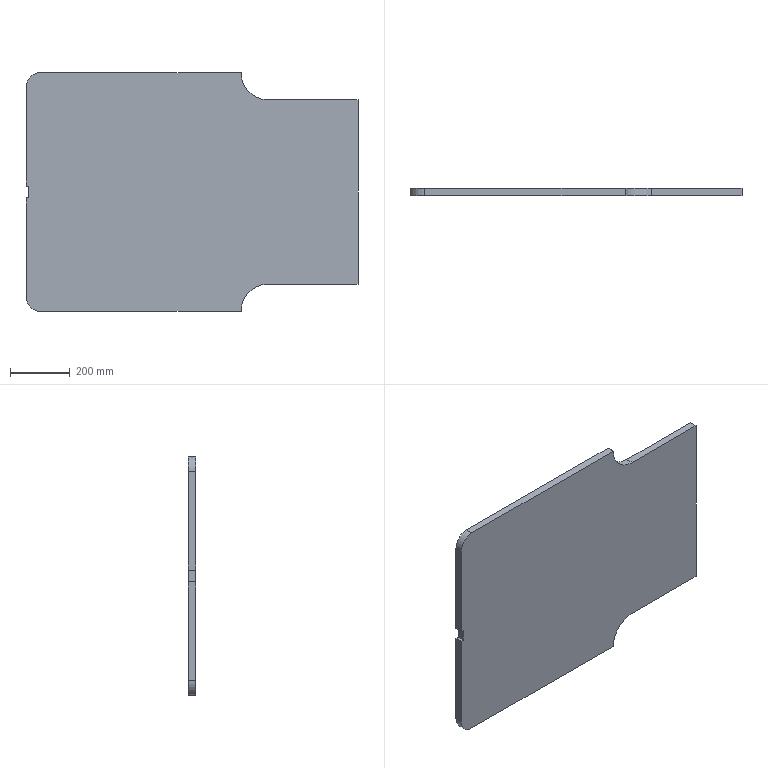Part | SolidWorks | features BaseBody 1 | 1 solid | 54 faces | box 1112 x 25 x 800 mm | volume 20489758 mm3 | cylinder 28 | plane 26 | commonest cylinder face diameters 10 x24 100 x2 178 x2
STEP:
#1=CARTESIAN_POINT('',(-375.282,-2.862,-275.));
#2=VERTEX_POINT('',#1);
#3=CARTESIAN_POINT('',(-375.282,-2.862,-265.));
#4=VERTEX_POINT('',#3);
#5=CARTESIAN_POINT('',(-375.282,-2.862,-270.));
#6=DIRECTION('',(0.,1.,0.));
#7=DIRECTION('',(0.,0.,1.));
#8=AXIS2_PLACEMENT_3D('',#5,#6,#7);
#9=CIRCLE('',#8,5.);
#10=EDGE_CURVE('',#2,#4,#9,.T.);
#11=ORIENTED_EDGE('',*,*,#10,.F.);
#12=CARTESIAN_POINT('',(-375.282,7.138,-275.));
#13=VERTEX_POINT('',#12);
#14=CARTESIAN_POINT('',(-375.282,-2.862,-275.));
#15=DIRECTION('',(0.,1.,0.));
#16=VECTOR('',#15,1000.);
#17=LINE('',#14,#16);
#18=EDGE_CURVE('',#2,#13,#17,.T.);
#19=ORIENTED_EDGE('',*,*,#18,.T.);
#20=CARTESIAN_POINT('',(-375.282,7.138,-265.));
#21=VERTEX_POINT('',#20);
#22=CARTESIAN_POINT('',(-375.282,7.138,-270.));
#23=DIRECTION('',(0.,-1.,0.));
#24=DIRECTION('',(0.,0.,1.));
#25=AXIS2_PLACEMENT_3D('',#22,#23,#24);
#26=CIRCLE('',#25,5.);
#27=EDGE_CURVE('',#21,#13,#26,.T.);
#28=ORIENTED_EDGE('',*,*,#27,.F.);
#29=CARTESIAN_POINT('',(-375.282,-2.862,-265.));
#30=DIRECTION('',(0.,1.,0.));
#31=VECTOR('',#30,1000.);
#32=LINE('',#29,#31);
#33=EDGE_CURVE('',#4,#21,#32,.T.);
#34=ORIENTED_EDGE('',*,*,#33,.F.);
#35=EDGE_LOOP('',(#11,#19,#28,#34));
#36=FACE_OUTER_BOUND('',#35,.T.);
#37=CARTESIAN_POINT('',(-375.282,-2.862,-270.));
#38=DIRECTION('',(0.,1.,0.));
#39=DIRECTION('',(0.,0.,1.));
#40=AXIS2_PLACEMENT_3D('',#37,#38,#39);
#41=CYLINDRICAL_SURFACE('',#40,5.);
#42=ADVANCED_FACE('',(#36),#41,.F.);
#43=CARTESIAN_POINT('',(-510.782,-2.862,-275.));
#44=VERTEX_POINT('',#43);
#45=CARTESIAN_POINT('',(-510.782,-2.862,-265.));
#46=VERTEX_POINT('',#45);
#47=CARTESIAN_POINT('',(-510.782,-2.862,-270.));
#48=DIRECTION('',(0.,1.,0.));
#49=DIRECTION('',(0.,0.,1.));
#50=AXIS2_PLACEMENT_3D('',#47,#48,#49);
#51=CIRCLE('',#50,5.);
#52=EDGE_CURVE('',#44,#46,#51,.T.);
#53=ORIENTED_EDGE('',*,*,#52,.F.);
#54=CARTESIAN_POINT('',(-510.782,7.138,-275.));
#55=VERTEX_POINT('',#54);
#56=CARTESIAN_POINT('',(-510.782,-2.862,-275.));
#57=DIRECTION('',(0.,1.,0.));
#58=VECTOR('',#57,1000.);
#59=LINE('',#56,#58);
#60=EDGE_CURVE('',#44,#55,#59,.T.);
#61=ORIENTED_EDGE('',*,*,#60,.T.);
#62=CARTESIAN_POINT('',(-510.782,7.138,-265.));
#63=VERTEX_POINT('',#62);
#64=CARTESIAN_POINT('',(-510.782,7.138,-270.));
#65=DIRECTION('',(0.,-1.,0.));
#66=DIRECTION('',(0.,0.,1.));
#67=AXIS2_PLACEMENT_3D('',#64,#65,#66);
#68=CIRCLE('',#67,5.);
#69=EDGE_CURVE('',#63,#55,#68,.T.);
#70=ORIENTED_EDGE('',*,*,#69,.F.);
#71=CARTESIAN_POINT('',(-510.782,-2.862,-265.));
#72=DIRECTION('',(0.,1.,0.));
#73=VECTOR('',#72,1000.);
#74=LINE('',#71,#73);
#75=EDGE_CURVE('',#46,#63,#74,.T.);
#76=ORIENTED_EDGE('',*,*,#75,.F.);
#77=EDGE_LOOP('',(#53,#61,#70,#76));
#78=FACE_OUTER_BOUND('',#77,.T.);
#79=CARTESIAN_POINT('',(-510.782,-2.862,-270.));
#80=DIRECTION('',(0.,1.,0.));
#81=DIRECTION('',(0.,0.,1.));
#82=AXIS2_PLACEMENT_3D('',#79,#80,#81);
#83=CYLINDRICAL_SURFACE('',#82,5.);
#84=ADVANCED_FACE('',(#78),#83,.F.);
#85=CARTESIAN_POINT('',(418.218,-2.862,-285.));
#86=VERTEX_POINT('',#85);
#87=CARTESIAN_POINT('',(418.218,-2.862,-275.));
#88=VERTEX_POINT('',#87);
#89=CARTESIAN_POINT('',(418.218,-2.862,-280.));
#90=DIRECTION('',(0.,1.,0.));
#91=DIRECTION('',(0.,0.,1.));
#92=AXIS2_PLACEMENT_3D('',#89,#90,#91);
#93=CIRCLE('',#92,5.);
#94=EDGE_CURVE('',#86,#88,#93,.T.);
#95=ORIENTED_EDGE('',*,*,#94,.F.);
#96=CARTESIAN_POINT('',(418.218,7.138,-285.));
#97=VERTEX_POINT('',#96);
#98=CARTESIAN_POINT('',(418.218,-2.862,-285.));
#99=DIRECTION('',(0.,1.,0.));
#100=VECTOR('',#99,1000.);
#101=LINE('',#98,#100);
#102=EDGE_CURVE('',#86,#97,#101,.T.);
#103=ORIENTED_EDGE('',*,*,#102,.T.);
#104=CARTESIAN_POINT('',(418.218,7.138,-275.));
#105=VERTEX_POINT('',#104);
#106=CARTESIAN_POINT('',(418.218,7.138,-280.));
#107=DIRECTION('',(0.,-1.,0.));
#108=DIRECTION('',(0.,0.,1.));
#109=AXIS2_PLACEMENT_3D('',#106,#107,#108);
#110=CIRCLE('',#109,5.);
#111=EDGE_CURVE('',#105,#97,#110,.T.);
#112=ORIENTED_EDGE('',*,*,#111,.F.);
#113=CARTESIAN_POINT('',(418.218,-2.862,-275.));
#114=DIRECTION('',(0.,1.,0.));
#115=VECTOR('',#114,1000.);
#116=LINE('',#113,#115);
#117=EDGE_CURVE('',#88,#105,#116,.T.);
#118=ORIENTED_EDGE('',*,*,#117,.F.);
#119=EDGE_LOOP('',(#95,#103,#112,#118));
#120=FACE_OUTER_BOUND('',#119,.T.);
#121=CARTESIAN_POINT('',(418.218,-2.862,-280.));
#122=DIRECTION('',(0.,1.,0.));
#123=DIRECTION('',(0.,0.,1.));
#124=AXIS2_PLACEMENT_3D('',#121,#122,#123);
#125=CYLINDRICAL_SURFACE('',#124,5.);
#126=ADVANCED_FACE('',(#120),#125,.F.);
#127=CARTESIAN_POINT('',(299.701,-2.862,-285.));
#128=VERTEX_POINT('',#127);
#129=CARTESIAN_POINT('',(299.701,-2.862,-275.));
#130=VERTEX_POINT('',#129);
#131=CARTESIAN_POINT('',(299.701,-2.862,-280.));
#132=DIRECTION('',(0.,1.,0.));
#133=DIRECTION('',(0.,0.,1.));
#134=AXIS2_PLACEMENT_3D('',#131,#132,#133);
#135=CIRCLE('',#134,5.);
#136=EDGE_CURVE('',#128,#130,#135,.T.);
#137=ORIENTED_EDGE('',*,*,#136,.F.);
#138=CARTESIAN_POINT('',(299.701,7.138,-285.));
#139=VERTEX_POINT('',#138);
#140=CARTESIAN_POINT('',(299.701,-2.862,-285.));
#141=DIRECTION('',(0.,1.,0.));
#142=VECTOR('',#141,1000.);
#143=LINE('',#140,#142);
#144=EDGE_CURVE('',#128,#139,#143,.T.);
#145=ORIENTED_EDGE('',*,*,#144,.T.);
#146=CARTESIAN_POINT('',(299.701,7.138,-275.));
#147=VERTEX_POINT('',#146);
#148=CARTESIAN_POINT('',(299.701,7.138,-280.));
#149=DIRECTION('',(0.,-1.,0.));
#150=DIRECTION('',(0.,0.,1.));
#151=AXIS2_PLACEMENT_3D('',#148,#149,#150);
#152=CIRCLE('',#151,5.);
#153=EDGE_CURVE('',#147,#139,#152,.T.);
#154=ORIENTED_EDGE('',*,*,#153,.F.);
#155=CARTESIAN_POINT('',(299.701,-2.862,-275.));
#156=DIRECTION('',(0.,1.,0.));
#157=VECTOR('',#156,1000.);
#158=LINE('',#155,#157);
#159=EDGE_CURVE('',#130,#147,#158,.T.);
#160=ORIENTED_EDGE('',*,*,#159,.F.);
#161=EDGE_LOOP('',(#137,#145,#154,#160));
#162=FACE_OUTER_BOUND('',#161,.T.);
#163=CARTESIAN_POINT('',(299.701,-2.862,-280.));
#164=DIRECTION('',(0.,1.,0.));
#165=DIRECTION('',(0.,0.,1.));
#166=AXIS2_PLACEMENT_3D('',#163,#164,#165);
#167=CYLINDRICAL_SURFACE('',#166,5.);
#168=ADVANCED_FACE('',(#162),#167,.F.);
#169=CARTESIAN_POINT('',(418.218,-2.862,275.));
#170=VERTEX_POINT('',#169);
#171=CARTESIAN_POINT('',(418.218,-2.862,285.));
#172=VERTEX_POINT('',#171);
#173=CARTESIAN_POINT('',(418.218,-2.862,280.));
#174=DIRECTION('',(0.,1.,0.));
#175=DIRECTION('',(0.,0.,-1.));
#176=AXIS2_PLACEMENT_3D('',#173,#174,#175);
#177=CIRCLE('',#176,5.);
#178=EDGE_CURVE('',#170,#172,#177,.T.);
#179=ORIENTED_EDGE('',*,*,#178,.F.);
#180=CARTESIAN_POINT('',(418.218,7.138,275.));
#181=VERTEX_POINT('',#180);
#182=CARTESIAN_POINT('',(418.218,-2.862,275.));
#183=DIRECTION('',(0.,1.,0.));
#184=VECTOR('',#183,1000.);
#185=LINE('',#182,#184);
#186=EDGE_CURVE('',#170,#181,#185,.T.);
#187=ORIENTED_EDGE('',*,*,#186,.T.);
#188=CARTESIAN_POINT('',(418.218,7.138,285.));
#189=VERTEX_POINT('',#188);
#190=CARTESIAN_POINT('',(418.218,7.138,280.));
#191=DIRECTION('',(0.,-1.,0.));
#192=DIRECTION('',(0.,0.,1.));
#193=AXIS2_PLACEMENT_3D('',#190,#191,#192);
#194=CIRCLE('',#193,5.);
#195=EDGE_CURVE('',#189,#181,#194,.T.);
#196=ORIENTED_EDGE('',*,*,#195,.F.);
#197=CARTESIAN_POINT('',(418.218,-2.862,285.));
#198=DIRECTION('',(0.,1.,0.));
#199=VECTOR('',#198,1000.);
#200=LINE('',#197,#199);
#201=EDGE_CURVE('',#172,#189,#200,.T.);
#202=ORIENTED_EDGE('',*,*,#201,.F.);
#203=EDGE_LOOP('',(#179,#187,#196,#202));
#204=FACE_OUTER_BOUND('',#203,.T.);
#205=CARTESIAN_POINT('',(418.218,-2.862,280.));
#206=DIRECTION('',(0.,1.,0.));
#207=DIRECTION('',(0.,0.,1.));
#208=AXIS2_PLACEMENT_3D('',#205,#206,#207);
#209=CYLINDRICAL_SURFACE('',#208,5.);
#210=ADVANCED_FACE('',(#204),#209,.F.);
#211=CARTESIAN_POINT('',(299.701,-2.862,275.));
#212=VERTEX_POINT('',#211);
#213=CARTESIAN_POINT('',(299.701,-2.862,285.));
#214=VERTEX_POINT('',#213);
#215=CARTESIAN_POINT('',(299.701,-2.862,280.));
#216=DIRECTION('',(0.,1.,0.));
#217=DIRECTION('',(0.,0.,-1.));
#218=AXIS2_PLACEMENT_3D('',#215,#216,#217);
#219=CIRCLE('',#218,5.);
#220=EDGE_CURVE('',#212,#214,#219,.T.);
#221=ORIENTED_EDGE('',*,*,#220,.F.);
#222=CARTESIAN_POINT('',(299.701,7.138,275.));
#223=VERTEX_POINT('',#222);
#224=CARTESIAN_POINT('',(299.701,-2.862,275.));
#225=DIRECTION('',(0.,1.,0.));
#226=VECTOR('',#225,1000.);
#227=LINE('',#224,#226);
#228=EDGE_CURVE('',#212,#223,#227,.T.);
#229=ORIENTED_EDGE('',*,*,#228,.T.);
#230=CARTESIAN_POINT('',(299.701,7.138,285.));
#231=VERTEX_POINT('',#230);
#232=CARTESIAN_POINT('',(299.701,7.138,280.));
#233=DIRECTION('',(0.,-1.,0.));
#234=DIRECTION('',(0.,0.,1.));
#235=AXIS2_PLACEMENT_3D('',#232,#233,#234);
#236=CIRCLE('',#235,5.);
#237=EDGE_CURVE('',#231,#223,#236,.T.);
#238=ORIENTED_EDGE('',*,*,#237,.F.);
#239=CARTESIAN_POINT('',(299.701,-2.862,285.));
#240=DIRECTION('',(0.,1.,0.));
#241=VECTOR('',#240,1000.);
#242=LINE('',#239,#241);
#243=EDGE_CURVE('',#214,#231,#242,.T.);
#244=ORIENTED_EDGE('',*,*,#243,.F.);
#245=EDGE_LOOP('',(#221,#229,#238,#244));
#246=FACE_OUTER_BOUND('',#245,.T.);
#247=CARTESIAN_POINT('',(299.701,-2.862,280.));
#248=DIRECTION('',(0.,1.,0.));
#249=DIRECTION('',(0.,0.,1.));
#250=AXIS2_PLACEMENT_3D('',#247,#248,#249);
#251=CYLINDRICAL_SURFACE('',#250,5.);
#252=ADVANCED_FACE('',(#246),#251,.F.);
#253=CARTESIAN_POINT('',(-375.282,-2.862,265.));
#254=VERTEX_POINT('',#253);
#255=CARTESIAN_POINT('',(-375.282,-2.862,275.));
#256=VERTEX_POINT('',#255);
#257=CARTESIAN_POINT('',(-375.282,-2.862,270.));
#258=DIRECTION('',(0.,1.,0.));
#259=DIRECTION('',(0.,0.,-1.));
#260=AXIS2_PLACEMENT_3D('',#257,#258,#259);
#261=CIRCLE('',#260,5.);
#262=EDGE_CURVE('',#254,#256,#261,.T.);
#263=ORIENTED_EDGE('',*,*,#262,.F.);
#264=CARTESIAN_POINT('',(-375.282,7.138,265.));
#265=VERTEX_POINT('',#264);
#266=CARTESIAN_POINT('',(-375.282,-2.862,265.));
#267=DIRECTION('',(0.,1.,0.));
#268=VECTOR('',#267,1000.);
#269=LINE('',#266,#268);
#270=EDGE_CURVE('',#254,#265,#269,.T.);
#271=ORIENTED_EDGE('',*,*,#270,.T.);
#272=CARTESIAN_POINT('',(-375.282,7.138,275.));
#273=VERTEX_POINT('',#272);
#274=CARTESIAN_POINT('',(-375.282,7.138,270.));
#275=DIRECTION('',(0.,-1.,0.));
#276=DIRECTION('',(0.,0.,1.));
#277=AXIS2_PLACEMENT_3D('',#274,#275,#276);
#278=CIRCLE('',#277,5.);
#279=EDGE_CURVE('',#273,#265,#278,.T.);
#280=ORIENTED_EDGE('',*,*,#279,.F.);
#281=CARTESIAN_POINT('',(-375.282,-2.862,275.));
#282=DIRECTION('',(0.,1.,0.));
#283=VECTOR('',#282,1000.);
#284=LINE('',#281,#283);
#285=EDGE_CURVE('',#256,#273,#284,.T.);
#286=ORIENTED_EDGE('',*,*,#285,.F.);
#287=EDGE_LOOP('',(#263,#271,#280,#286));
#288=FACE_OUTER_BOUND('',#287,.T.);
#289=CARTESIAN_POINT('',(-375.282,-2.862,270.));
#290=DIRECTION('',(0.,1.,0.));
#291=DIRECTION('',(0.,0.,1.));
#292=AXIS2_PLACEMENT_3D('',#289,#290,#291);
#293=CYLINDRICAL_SURFACE('',#292,5.);
#294=ADVANCED_FACE('',(#288),#293,.F.);
#295=CARTESIAN_POINT('',(-510.782,-2.862,265.));
#296=VERTEX_POINT('',#295);
#297=CARTESIAN_POINT('',(-510.782,-2.862,275.));
#298=VERTEX_POINT('',#297);
#299=CARTESIAN_POINT('',(-510.782,-2.862,270.));
#300=DIRECTION('',(0.,1.,0.));
#301=DIRECTION('',(0.,0.,-1.));
#302=AXIS2_PLACEMENT_3D('',#299,#300,#301);
#303=CIRCLE('',#302,5.);
#304=EDGE_CURVE('',#296,#298,#303,.T.);
#305=ORIENTED_EDGE('',*,*,#304,.F.);
#306=CARTESIAN_POINT('',(-510.782,7.138,265.));
#307=VERTEX_POINT('',#306);
#308=CARTESIAN_POINT('',(-510.782,-2.862,265.));
#309=DIRECTION('',(0.,1.,0.));
#310=VECTOR('',#309,1000.);
#311=LINE('',#308,#310);
#312=EDGE_CURVE('',#296,#307,#311,.T.);
#313=ORIENTED_EDGE('',*,*,#312,.T.);
#314=CARTESIAN_POINT('',(-510.782,7.138,275.));
#315=VERTEX_POINT('',#314);
#316=CARTESIAN_POINT('',(-510.782,7.138,270.));
#317=DIRECTION('',(0.,-1.,0.));
#318=DIRECTION('',(0.,0.,1.));
#319=AXIS2_PLACEMENT_3D('',#316,#317,#318);
#320=CIRCLE('',#319,5.);
#321=EDGE_CURVE('',#315,#307,#320,.T.);
#322=ORIENTED_EDGE('',*,*,#321,.F.);
#323=CARTESIAN_POINT('',(-510.782,-2.862,275.));
#324=DIRECTION('',(0.,1.,0.));
#325=VECTOR('',#324,1000.);
#326=LINE('',#323,#325);
#327=EDGE_CURVE('',#298,#315,#326,.T.);
#328=ORIENTED_EDGE('',*,*,#327,.F.);
#329=EDGE_LOOP('',(#305,#313,#322,#328));
#330=FACE_OUTER_BOUND('',#329,.T.);
#331=CARTESIAN_POINT('',(-510.782,-2.862,270.));
#332=DIRECTION('',(0.,1.,0.));
#333=DIRECTION('',(0.,0.,1.));
#334=AXIS2_PLACEMENT_3D('',#331,#332,#333);
#335=CYLINDRICAL_SURFACE('',#334,5.);
#336=ADVANCED_FACE('',(#330),#335,.F.);
#337=CARTESIAN_POINT('',(-246.782,-2.862,105.));
#338=VERTEX_POINT('',#337);
#339=CARTESIAN_POINT('',(-246.782,-2.862,115.));
#340=VERTEX_POINT('',#339);
#341=CARTESIAN_POINT('',(-246.782,-2.862,110.));
#342=DIRECTION('',(0.,1.,0.));
#343=DIRECTION('',(0.,0.,1.));
#344=AXIS2_PLACEMENT_3D('',#341,#342,#343);
#345=CIRCLE('',#344,5.);
#346=EDGE_CURVE('',#338,#340,#345,.T.);
#347=ORIENTED_EDGE('',*,*,#346,.F.);
#348=CARTESIAN_POINT('',(-246.782,7.138,105.));
#349=VERTEX_POINT('',#348);
#350=CARTESIAN_POINT('',(-246.782,-2.862,105.));
#351=DIRECTION('',(0.,1.,0.));
#352=VECTOR('',#351,1000.);
#353=LINE('',#350,#352);
#354=EDGE_CURVE('',#338,#349,#353,.T.);
#355=ORIENTED_EDGE('',*,*,#354,.T.);
#356=CARTESIAN_POINT('',(-246.782,7.138,115.));
#357=VERTEX_POINT('',#356);
#358=CARTESIAN_POINT('',(-246.782,7.138,110.));
#359=DIRECTION('',(0.,-1.,0.));
#360=DIRECTION('',(0.,0.,1.));
#361=AXIS2_PLACEMENT_3D('',#358,#359,#360);
#362=CIRCLE('',#361,5.);
#363=EDGE_CURVE('',#357,#349,#362,.T.);
#364=ORIENTED_EDGE('',*,*,#363,.F.);
#365=CARTESIAN_POINT('',(-246.782,-2.862,115.));
#366=DIRECTION('',(0.,1.,0.));
#367=VECTOR('',#366,1000.);
#368=LINE('',#365,#367);
#369=EDGE_CURVE('',#340,#357,#368,.T.);
#370=ORIENTED_EDGE('',*,*,#369,.F.);
#371=EDGE_LOOP('',(#347,#355,#364,#370));
#372=FACE_OUTER_BOUND('',#371,.T.);
#373=CARTESIAN_POINT('',(-246.782,-2.862,110.));
#374=DIRECTION('',(0.,1.,0.));
#375=DIRECTION('',(0.,0.,1.));
#376=AXIS2_PLACEMENT_3D('',#373,#374,#375);
#377=CYLINDRICAL_SURFACE('',#376,5.);
#378=ADVANCED_FACE('',(#372),#377,.F.);
#379=CARTESIAN_POINT('',(-246.782,-2.862,165.));
#380=VERTEX_POINT('',#379);
#381=CARTESIAN_POINT('',(-246.782,-2.862,175.));
#382=VERTEX_POINT('',#381);
#383=CARTESIAN_POINT('',(-246.782,-2.862,170.));
#384=DIRECTION('',(0.,1.,0.));
#385=DIRECTION('',(0.,0.,1.));
#386=AXIS2_PLACEMENT_3D('',#383,#384,#385);
#387=CIRCLE('',#386,5.);
#388=EDGE_CURVE('',#380,#382,#387,.T.);
#389=ORIENTED_EDGE('',*,*,#388,.F.);
#390=CARTESIAN_POINT('',(-246.782,7.138,165.));
#391=VERTEX_POINT('',#390);
#392=CARTESIAN_POINT('',(-246.782,-2.862,165.));
#393=DIRECTION('',(0.,1.,0.));
#394=VECTOR('',#393,1000.);
#395=LINE('',#392,#394);
#396=EDGE_CURVE('',#380,#391,#395,.T.);
#397=ORIENTED_EDGE('',*,*,#396,.T.);
#398=CARTESIAN_POINT('',(-246.782,7.138,175.));
#399=VERTEX_POINT('',#398);
#400=CARTESIAN_POINT('',(-246.782,7.138,170.));
#401=DIRECTION('',(0.,-1.,0.));
#402=DIRECTION('',(0.,0.,1.));
#403=AXIS2_PLACEMENT_3D('',#400,#401,#402);
#404=CIRCLE('',#403,5.);
#405=EDGE_CURVE('',#399,#391,#404,.T.);
#406=ORIENTED_EDGE('',*,*,#405,.F.);
#407=CARTESIAN_POINT('',(-246.782,-2.862,175.));
#408=DIRECTION('',(0.,1.,0.));
#409=VECTOR('',#408,1000.);
#410=LINE('',#407,#409);
#411=EDGE_CURVE('',#382,#399,#410,.T.);
#412=ORIENTED_EDGE('',*,*,#411,.F.);
#413=EDGE_LOOP('',(#389,#397,#406,#412));
#414=FACE_OUTER_BOUND('',#413,.T.);
#415=CARTESIAN_POINT('',(-246.782,-2.862,170.));
#416=DIRECTION('',(0.,1.,0.));
#417=DIRECTION('',(0.,0.,1.));
#418=AXIS2_PLACEMENT_3D('',#415,#416,#417);
#419=CYLINDRICAL_SURFACE('',#418,5.);
#420=ADVANCED_FACE('',(#414),#419,.F.);
#421=CARTESIAN_POINT('',(-306.782,-2.862,165.));
#422=VERTEX_POINT('',#421);
#423=CARTESIAN_POINT('',(-306.782,-2.862,175.));
#424=VERTEX_POINT('',#423);
#425=CARTESIAN_POINT('',(-306.782,-2.862,170.));
#426=DIRECTION('',(0.,1.,0.));
#427=DIRECTION('',(0.,0.,-1.));
#428=AXIS2_PLACEMENT_3D('',#425,#426,#427);
#429=CIRCLE('',#428,5.);
#430=EDGE_CURVE('',#422,#424,#429,.T.);
#431=ORIENTED_EDGE('',*,*,#430,.F.);
#432=CARTESIAN_POINT('',(-306.782,7.138,165.));
#433=VERTEX_POINT('',#432);
#434=CARTESIAN_POINT('',(-306.782,-2.862,165.));
#435=DIRECTION('',(0.,1.,0.));
#436=VECTOR('',#435,1000.);
#437=LINE('',#434,#436);
#438=EDGE_CURVE('',#422,#433,#437,.T.);
#439=ORIENTED_EDGE('',*,*,#438,.T.);
#440=CARTESIAN_POINT('',(-306.782,7.138,175.));
#441=VERTEX_POINT('',#440);
#442=CARTESIAN_POINT('',(-306.782,7.138,170.));
#443=DIRECTION('',(0.,-1.,0.));
#444=DIRECTION('',(0.,0.,1.));
#445=AXIS2_PLACEMENT_3D('',#442,#443,#444);
#446=CIRCLE('',#445,5.);
#447=EDGE_CURVE('',#441,#433,#446,.T.);
#448=ORIENTED_EDGE('',*,*,#447,.F.);
#449=CARTESIAN_POINT('',(-306.782,-2.862,175.));
#450=DIRECTION('',(0.,1.,0.));
#451=VECTOR('',#450,1000.);
#452=LINE('',#449,#451);
#453=EDGE_CURVE('',#424,#441,#452,.T.);
#454=ORIENTED_EDGE('',*,*,#453,.F.);
#455=EDGE_LOOP('',(#431,#439,#448,#454));
#456=FACE_OUTER_BOUND('',#455,.T.);
#457=CARTESIAN_POINT('',(-306.782,-2.862,170.));
#458=DIRECTION('',(0.,1.,0.));
#459=DIRECTION('',(0.,0.,1.));
#460=AXIS2_PLACEMENT_3D('',#457,#458,#459);
#461=CYLINDRICAL_SURFACE('',#460,5.);
#462=ADVANCED_FACE('',(#456),#461,.F.);
#463=CARTESIAN_POINT('',(-306.782,-2.862,105.));
#464=VERTEX_POINT('',#463);
#465=CARTESIAN_POINT('',(-306.782,-2.862,115.));
#466=VERTEX_POINT('',#465);
#467=CARTESIAN_POINT('',(-306.782,-2.862,110.));
#468=DIRECTION('',(0.,1.,0.));
#469=DIRECTION('',(0.,0.,-1.));
#470=AXIS2_PLACEMENT_3D('',#467,#468,#469);
#471=CIRCLE('',#470,5.);
#472=EDGE_CURVE('',#464,#466,#471,.T.);
#473=ORIENTED_EDGE('',*,*,#472,.F.);
#474=CARTESIAN_POINT('',(-306.782,7.138,105.));
#475=VERTEX_POINT('',#474);
#476=CARTESIAN_POINT('',(-306.782,-2.862,105.));
#477=DIRECTION('',(0.,1.,0.));
#478=VECTOR('',#477,1000.);
#479=LINE('',#476,#478);
#480=EDGE_CURVE('',#464,#475,#479,.T.);
#481=ORIENTED_EDGE('',*,*,#480,.T.);
#482=CARTESIAN_POINT('',(-306.782,7.138,115.));
#483=VERTEX_POINT('',#482);
#484=CARTESIAN_POINT('',(-306.782,7.138,110.));
#485=DIRECTION('',(0.,-1.,0.));
#486=DIRECTION('',(0.,0.,1.));
#487=AXIS2_PLACEMENT_3D('',#484,#485,#486);
#488=CIRCLE('',#487,5.);
#489=EDGE_CURVE('',#483,#475,#488,.T.);
#490=ORIENTED_EDGE('',*,*,#489,.F.);
#491=CARTESIAN_POINT('',(-306.782,-2.862,115.));
#492=DIRECTION('',(0.,1.,0.));
#493=VECTOR('',#492,1000.);
#494=LINE('',#491,#493);
#495=EDGE_CURVE('',#466,#483,#494,.T.);
#496=ORIENTED_EDGE('',*,*,#495,.F.);
#497=EDGE_LOOP('',(#473,#481,#490,#496));
#498=FACE_OUTER_BOUND('',#497,.T.);
#499=CARTESIAN_POINT('',(-306.782,-2.862,110.));
#500=DIRECTION('',(0.,1.,0.));
#501=DIRECTION('',(0.,0.,1.));
#502=AXIS2_PLACEMENT_3D('',#499,#500,#501);
#503=CYLINDRICAL_SURFACE('',#502,5.);
#504=ADVANCED_FACE('',(#498),#503,.F.);
#505=CARTESIAN_POINT('',(-606.782,-17.862,-20.));
#506=VERTEX_POINT('',#505);
#507=CARTESIAN_POINT('',(-616.782,-17.862,-20.));
#508=VERTEX_POINT('',#507);
#509=CARTESIAN_POINT('',(-606.782,-17.862,-20.));
#510=DIRECTION('',(-1.,0.,0.));
#511=VECTOR('',#510,1000.);
#512=LINE('',#509,#511);
#513=EDGE_CURVE('',#506,#508,#512,.T.);
#514=ORIENTED_EDGE('',*,*,#513,.T.);
#515=CARTESIAN_POINT('',(-616.782,-17.862,-350.));
#516=VERTEX_POINT('',#515);
#517=CARTESIAN_POINT('',(-616.782,-17.862,350.));
#518=DIRECTION('',(0.,0.,1.));
#519=VECTOR('',#518,1000.);
#520=LINE('',#517,#519);
#521=EDGE_CURVE('',#516,#508,#520,.T.);
#522=ORIENTED_EDGE('',*,*,#521,.F.);
#523=CARTESIAN_POINT('',(-566.782,-17.862,-400.));
#524=VERTEX_POINT('',#523);
#525=CARTESIAN_POINT('',(-566.782,-17.862,-350.));
#526=DIRECTION('',(0.,1.,0.));
#527=DIRECTION('',(0.,0.,-1.));
#528=AXIS2_PLACEMENT_3D('',#525,#526,#527);
#529=CIRCLE('',#528,50.);
#530=EDGE_CURVE('',#524,#516,#529,.T.);
#531=ORIENTED_EDGE('',*,*,#530,.F.);
#532=CARTESIAN_POINT('',(103.218,-17.862,-400.));
#533=VERTEX_POINT('',#532);
#534=CARTESIAN_POINT('',(-566.782,-17.862,-400.));
#535=DIRECTION('',(-1.,0.,0.));
#536=VECTOR('',#535,1000.);
#537=LINE('',#534,#536);
#538=EDGE_CURVE('',#533,#524,#537,.T.);
#539=ORIENTED_EDGE('',*,*,#538,.F.);
#540=CARTESIAN_POINT('',(103.218,-17.862,-398.));
#541=VERTEX_POINT('',#540);
#542=CARTESIAN_POINT('',(103.218,-17.862,-400.));
#543=DIRECTION('',(0.,0.,-1.));
#544=VECTOR('',#543,1000.);
#545=LINE('',#542,#544);
#546=EDGE_CURVE('',#541,#533,#545,.T.);
#547=ORIENTED_EDGE('',*,*,#546,.F.);
#548=CARTESIAN_POINT('',(192.218,-17.862,-309.));
#549=VERTEX_POINT('',#548);
#550=CARTESIAN_POINT('',(192.218,-17.862,-398.));
#551=DIRECTION('',(0.,-1.,0.));
#552=DIRECTION('',(0.,0.,-1.));
#553=AXIS2_PLACEMENT_3D('',#550,#551,#552);
#554=CIRCLE('',#553,89.);
#555=EDGE_CURVE('',#549,#541,#554,.T.);
#556=ORIENTED_EDGE('',*,*,#555,.F.);
#557=CARTESIAN_POINT('',(494.869,-17.862,-309.));
#558=VERTEX_POINT('',#557);
#559=CARTESIAN_POINT('',(192.218,-17.862,-309.));
#560=DIRECTION('',(-1.,0.,0.));
#561=VECTOR('',#560,1000.);
#562=LINE('',#559,#561);
#563=EDGE_CURVE('',#558,#549,#562,.T.);
#564=ORIENTED_EDGE('',*,*,#563,.F.);
#565=CARTESIAN_POINT('',(494.869,-17.862,309.));
#566=VERTEX_POINT('',#565);
#567=CARTESIAN_POINT('',(494.869,-17.862,-189.));
#568=DIRECTION('',(0.,0.,-1.));
#569=VECTOR('',#568,1000.);
#570=LINE('',#567,#569);
#571=EDGE_CURVE('',#566,#558,#570,.T.);
#572=ORIENTED_EDGE('',*,*,#571,.F.);
#573=CARTESIAN_POINT('',(192.218,-17.862,309.));
#574=VERTEX_POINT('',#573);
#575=CARTESIAN_POINT('',(192.218,-17.862,309.));
#576=DIRECTION('',(1.,0.,0.));
#577=VECTOR('',#576,1000.);
#578=LINE('',#575,#577);
#579=EDGE_CURVE('',#574,#566,#578,.T.);
#580=ORIENTED_EDGE('',*,*,#579,.F.);
#581=CARTESIAN_POINT('',(103.218,-17.862,398.));
#582=VERTEX_POINT('',#581);
#583=CARTESIAN_POINT('',(192.218,-17.862,398.));
#584=DIRECTION('',(0.,-1.,0.));
#585=DIRECTION('',(0.,0.,-1.));
#586=AXIS2_PLACEMENT_3D('',#583,#584,#585);
#587=CIRCLE('',#586,89.);
#588=EDGE_CURVE('',#582,#574,#587,.T.);
#589=ORIENTED_EDGE('',*,*,#588,.F.);
#590=CARTESIAN_POINT('',(103.218,-17.862,400.));
#591=VERTEX_POINT('',#590);
#592=CARTESIAN_POINT('',(103.218,-17.862,400.));
#593=DIRECTION('',(0.,0.,-1.));
#594=VECTOR('',#593,1000.);
#595=LINE('',#592,#594);
#596=EDGE_CURVE('',#591,#582,#595,.T.);
#597=ORIENTED_EDGE('',*,*,#596,.F.);
#598=CARTESIAN_POINT('',(-566.782,-17.862,400.));
#599=VERTEX_POINT('',#598);
#600=CARTESIAN_POINT('',(-566.782,-17.862,400.));
#601=DIRECTION('',(1.,0.,0.));
#602=VECTOR('',#601,1000.);
#603=LINE('',#600,#602);
#604=EDGE_CURVE('',#599,#591,#603,.T.);
#605=ORIENTED_EDGE('',*,*,#604,.F.);
#606=CARTESIAN_POINT('',(-616.782,-17.862,350.));
#607=VERTEX_POINT('',#606);
#608=CARTESIAN_POINT('',(-566.782,-17.862,350.));
#609=DIRECTION('',(0.,1.,0.));
#610=DIRECTION('',(0.,0.,-1.));
#611=AXIS2_PLACEMENT_3D('',#608,#609,#610);
#612=CIRCLE('',#611,50.);
#613=EDGE_CURVE('',#607,#599,#612,.T.);
#614=ORIENTED_EDGE('',*,*,#613,.F.);
#615=CARTESIAN_POINT('',(-616.782,-17.862,20.));
#616=VERTEX_POINT('',#615);
#617=CARTESIAN_POINT('',(-616.782,-17.862,350.));
#618=DIRECTION('',(0.,0.,1.));
#619=VECTOR('',#618,1000.);
#620=LINE('',#617,#619);
#621=EDGE_CURVE('',#616,#607,#620,.T.);
#622=ORIENTED_EDGE('',*,*,#621,.F.);
#623=CARTESIAN_POINT('',(-606.782,-17.862,20.));
#624=VERTEX_POINT('',#623);
#625=CARTESIAN_POINT('',(-606.782,-17.862,20.));
#626=DIRECTION('',(-1.,0.,0.));
#627=VECTOR('',#626,1000.);
#628=LINE('',#625,#627);
#629=EDGE_CURVE('',#624,#616,#628,.T.);
#630=ORIENTED_EDGE('',*,*,#629,.F.);
#631=CARTESIAN_POINT('',(-606.782,-17.862,20.));
#632=DIRECTION('',(0.,0.,1.));
#633=VECTOR('',#632,1000.);
#634=LINE('',#631,#633);
#635=EDGE_CURVE('',#506,#624,#634,.T.);
#636=ORIENTED_EDGE('',*,*,#635,.F.);
#637=EDGE_LOOP('',(#514,#522,#531,#539,#547,#556,#564,#572,#580,#589,#597,#605,#614,#622,#630,#636));
#638=FACE_OUTER_BOUND('',#637,.T.);
#639=CARTESIAN_POINT('',(192.218,-17.862,-398.));
#640=DIRECTION('',(0.,-1.,0.));
#641=DIRECTION('',(0.,0.,-1.));
#642=AXIS2_PLACEMENT_3D('',#639,#640,#641);
#643=PLANE('',#642);
#644=ADVANCED_FACE('',(#638),#643,.T.);
#645=ORIENTED_EDGE('',*,*,#588,.T.);
#646=CARTESIAN_POINT('',(192.218,7.138,309.));
#647=VERTEX_POINT('',#646);
#648=CARTESIAN_POINT('',(192.218,7.138,309.));
#649=DIRECTION('',(0.,-1.,0.));
#650=VECTOR('',#649,1000.);
#651=LINE('',#648,#650);
#652=EDGE_CURVE('',#647,#574,#651,.T.);
#653=ORIENTED_EDGE('',*,*,#652,.F.);
#654=CARTESIAN_POINT('',(103.218,7.138,398.));
#655=VERTEX_POINT('',#654);
#656=CARTESIAN_POINT('',(192.218,7.138,398.));
#657=DIRECTION('',(0.,-1.,0.));
#658=DIRECTION('',(0.,0.,-1.));
#659=AXIS2_PLACEMENT_3D('',#656,#657,#658);
#660=CIRCLE('',#659,89.);
#661=EDGE_CURVE('',#655,#647,#660,.T.);
#662=ORIENTED_EDGE('',*,*,#661,.F.);
#663=CARTESIAN_POINT('',(103.218,7.138,398.));
#664=DIRECTION('',(0.,-1.,0.));
#665=VECTOR('',#664,1000.);
#666=LINE('',#663,#665);
#667=EDGE_CURVE('',#655,#582,#666,.T.);
#668=ORIENTED_EDGE('',*,*,#667,.T.);
#669=EDGE_LOOP('',(#645,#653,#662,#668));
#670=FACE_OUTER_BOUND('',#669,.T.);
#671=CARTESIAN_POINT('',(192.218,7.138,398.));
#672=DIRECTION('',(0.,-1.,0.));
#673=DIRECTION('',(0.,0.,-1.));
#674=AXIS2_PLACEMENT_3D('',#671,#672,#673);
#675=CYLINDRICAL_SURFACE('',#674,89.);
#676=ADVANCED_FACE('',(#670),#675,.F.);
#677=ORIENTED_EDGE('',*,*,#596,.T.);
#678=ORIENTED_EDGE('',*,*,#667,.F.);
#679=CARTESIAN_POINT('',(103.218,7.138,400.));
#680=VERTEX_POINT('',#679);
#681=CARTESIAN_POINT('',(103.218,7.138,400.));
#682=DIRECTION('',(0.,0.,-1.));
#683=VECTOR('',#682,1000.);
#684=LINE('',#681,#683);
#685=EDGE_CURVE('',#680,#655,#684,.T.);
#686=ORIENTED_EDGE('',*,*,#685,.F.);
#687=CARTESIAN_POINT('',(103.218,7.138,400.));
#688=DIRECTION('',(0.,-1.,0.));
#689=VECTOR('',#688,1000.);
#690=LINE('',#687,#689);
#691=EDGE_CURVE('',#680,#591,#690,.T.);
#692=ORIENTED_EDGE('',*,*,#691,.T.);
#693=EDGE_LOOP('',(#677,#678,#686,#692));
#694=FACE_OUTER_BOUND('',#693,.T.);
#695=CARTESIAN_POINT('',(103.218,7.138,400.));
#696=DIRECTION('',(-1.,0.,0.));
#697=DIRECTION('',(0.,0.,1.));
#698=AXIS2_PLACEMENT_3D('',#695,#696,#697);
#699=PLANE('',#698);
#700=ADVANCED_FACE('',(#694),#699,.F.);
#701=ORIENTED_EDGE('',*,*,#604,.T.);
#702=ORIENTED_EDGE('',*,*,#691,.F.);
#703=CARTESIAN_POINT('',(-566.782,7.138,400.));
#704=VERTEX_POINT('',#703);
#705=CARTESIAN_POINT('',(-566.782,7.138,400.));
#706=DIRECTION('',(1.,0.,0.));
#707=VECTOR('',#706,1000.);
#708=LINE('',#705,#707);
#709=EDGE_CURVE('',#704,#680,#708,.T.);
#710=ORIENTED_EDGE('',*,*,#709,.F.);
#711=CARTESIAN_POINT('',(-566.782,7.138,400.));
#712=DIRECTION('',(0.,-1.,0.));
#713=VECTOR('',#712,1000.);
#714=LINE('',#711,#713);
#715=EDGE_CURVE('',#704,#599,#714,.T.);
#716=ORIENTED_EDGE('',*,*,#715,.T.);
#717=EDGE_LOOP('',(#701,#702,#710,#716));
#718=FACE_OUTER_BOUND('',#717,.T.);
#719=CARTESIAN_POINT('',(-566.782,7.138,400.));
#720=DIRECTION('',(0.,0.,-1.));
#721=DIRECTION('',(-1.,0.,0.));
#722=AXIS2_PLACEMENT_3D('',#719,#720,#721);
#723=PLANE('',#722);
#724=ADVANCED_FACE('',(#718),#723,.F.);
#725=ORIENTED_EDGE('',*,*,#613,.T.);
#726=ORIENTED_EDGE('',*,*,#715,.F.);
#727=CARTESIAN_POINT('',(-616.782,7.138,350.));
#728=VERTEX_POINT('',#727);
#729=CARTESIAN_POINT('',(-566.782,7.138,350.));
#730=DIRECTION('',(0.,1.,0.));
#731=DIRECTION('',(0.,0.,-1.));
#732=AXIS2_PLACEMENT_3D('',#729,#730,#731);
#733=CIRCLE('',#732,50.);
#734=EDGE_CURVE('',#728,#704,#733,.T.);
#735=ORIENTED_EDGE('',*,*,#734,.F.);
#736=CARTESIAN_POINT('',(-616.782,7.138,350.));
#737=DIRECTION('',(0.,-1.,0.));
#738=VECTOR('',#737,1000.);
#739=LINE('',#736,#738);
#740=EDGE_CURVE('',#728,#607,#739,.T.);
#741=ORIENTED_EDGE('',*,*,#740,.T.);
#742=EDGE_LOOP('',(#725,#726,#735,#741));
#743=FACE_OUTER_BOUND('',#742,.T.);
#744=CARTESIAN_POINT('',(-566.782,7.138,350.));
#745=DIRECTION('',(0.,-1.,0.));
#746=DIRECTION('',(0.,0.,-1.));
#747=AXIS2_PLACEMENT_3D('',#744,#745,#746);
#748=CYLINDRICAL_SURFACE('',#747,50.);
#749=ADVANCED_FACE('',(#743),#748,.T.);
#750=CARTESIAN_POINT('',(-616.782,7.138,20.));
#751=VERTEX_POINT('',#750);
#752=CARTESIAN_POINT('',(-616.782,7.138,350.));
#753=DIRECTION('',(0.,0.,1.));
#754=VECTOR('',#753,1000.);
#755=LINE('',#752,#754);
#756=EDGE_CURVE('',#751,#728,#755,.T.);
#757=ORIENTED_EDGE('',*,*,#756,.F.);
#758=CARTESIAN_POINT('',(-616.782,7.138,20.));
#759=DIRECTION('',(0.,1.,0.));
#760=VECTOR('',#759,1000.);
#761=LINE('',#758,#760);
#762=EDGE_CURVE('',#616,#751,#761,.T.);
#763=ORIENTED_EDGE('',*,*,#762,.F.);
#764=ORIENTED_EDGE('',*,*,#621,.T.);
#765=ORIENTED_EDGE('',*,*,#740,.F.);
#766=EDGE_LOOP('',(#757,#763,#764,#765));
#767=FACE_OUTER_BOUND('',#766,.T.);
#768=CARTESIAN_POINT('',(-616.782,7.138,350.));
#769=DIRECTION('',(1.,0.,0.));
#770=DIRECTION('',(0.,0.,-1.));
#771=AXIS2_PLACEMENT_3D('',#768,#769,#770);
#772=PLANE('',#771);
#773=ADVANCED_FACE('',(#767),#772,.F.);
#774=ORIENTED_EDGE('',*,*,#762,.T.);
#775=CARTESIAN_POINT('',(-606.782,7.138,20.));
#776=VERTEX_POINT('',#775);
#777=CARTESIAN_POINT('',(-606.782,7.138,20.));
#778=DIRECTION('',(-1.,0.,0.));
#779=VECTOR('',#778,1000.);
#780=LINE('',#777,#779);
#781=EDGE_CURVE('',#776,#751,#780,.T.);
#782=ORIENTED_EDGE('',*,*,#781,.F.);
#783=CARTESIAN_POINT('',(-606.782,7.138,20.));
#784=DIRECTION('',(0.,1.,0.));
#785=VECTOR('',#784,1000.);
#786=LINE('',#783,#785);
#787=EDGE_CURVE('',#624,#776,#786,.T.);
#788=ORIENTED_EDGE('',*,*,#787,.F.);
#789=ORIENTED_EDGE('',*,*,#629,.T.);
#790=EDGE_LOOP('',(#774,#782,#788,#789));
#791=FACE_OUTER_BOUND('',#790,.T.);
#792=CARTESIAN_POINT('',(-606.782,7.138,20.));
#793=DIRECTION('',(0.,0.,1.));
#794=DIRECTION('',(0.,-1.,0.));
#795=AXIS2_PLACEMENT_3D('',#792,#793,#794);
#796=PLANE('',#795);
#797=ADVANCED_FACE('',(#791),#796,.F.);
#798=ORIENTED_EDGE('',*,*,#635,.T.);
#799=ORIENTED_EDGE('',*,*,#787,.T.);
#800=CARTESIAN_POINT('',(-606.782,7.138,-20.));
#801=VERTEX_POINT('',#800);
#802=CARTESIAN_POINT('',(-606.782,7.138,-20.));
#803=DIRECTION('',(0.,0.,-1.));
#804=VECTOR('',#803,1000.);
#805=LINE('',#802,#804);
#806=EDGE_CURVE('',#776,#801,#805,.T.);
#807=ORIENTED_EDGE('',*,*,#806,.T.);
#808=CARTESIAN_POINT('',(-606.782,-17.862,-20.));
#809=DIRECTION('',(0.,-1.,0.));
#810=VECTOR('',#809,1000.);
#811=LINE('',#808,#810);
#812=EDGE_CURVE('',#801,#506,#811,.T.);
#813=ORIENTED_EDGE('',*,*,#812,.T.);
#814=EDGE_LOOP('',(#798,#799,#807,#813));
#815=FACE_OUTER_BOUND('',#814,.T.);
#816=CARTESIAN_POINT('',(-606.782,-17.862,0.));
#817=DIRECTION('',(1.,0.,0.));
#818=DIRECTION('',(0.,0.,-1.));
#819=AXIS2_PLACEMENT_3D('',#816,#817,#818);
#820=PLANE('',#819);
#821=ADVANCED_FACE('',(#815),#820,.F.);
#822=CARTESIAN_POINT('',(-616.782,7.138,-20.));
#823=VERTEX_POINT('',#822);
#824=CARTESIAN_POINT('',(-616.782,-17.862,-20.));
#825=DIRECTION('',(0.,-1.,0.));
#826=VECTOR('',#825,1000.);
#827=LINE('',#824,#826);
#828=EDGE_CURVE('',#823,#508,#827,.T.);
#829=ORIENTED_EDGE('',*,*,#828,.T.);
#830=ORIENTED_EDGE('',*,*,#513,.F.);
#831=ORIENTED_EDGE('',*,*,#812,.F.);
#832=CARTESIAN_POINT('',(-606.782,7.138,-20.));
#833=DIRECTION('',(-1.,0.,0.));
#834=VECTOR('',#833,1000.);
#835=LINE('',#832,#834);
#836=EDGE_CURVE('',#801,#823,#835,.T.);
#837=ORIENTED_EDGE('',*,*,#836,.T.);
#838=EDGE_LOOP('',(#829,#830,#831,#837));
#839=FACE_OUTER_BOUND('',#838,.T.);
#840=CARTESIAN_POINT('',(-606.782,-17.862,-20.));
#841=DIRECTION('',(0.,0.,-1.));
#842=DIRECTION('',(0.,1.,0.));
#843=AXIS2_PLACEMENT_3D('',#840,#841,#842);
#844=PLANE('',#843);
#845=ADVANCED_FACE('',(#839),#844,.F.);
#846=ORIENTED_EDGE('',*,*,#521,.T.);
#847=ORIENTED_EDGE('',*,*,#828,.F.);
#848=CARTESIAN_POINT('',(-616.782,7.138,-350.));
#849=VERTEX_POINT('',#848);
#850=CARTESIAN_POINT('',(-616.782,7.138,350.));
#851=DIRECTION('',(0.,0.,1.));
#852=VECTOR('',#851,1000.);
#853=LINE('',#850,#852);
#854=EDGE_CURVE('',#849,#823,#853,.T.);
#855=ORIENTED_EDGE('',*,*,#854,.F.);
#856=CARTESIAN_POINT('',(-616.782,7.138,-350.));
#857=DIRECTION('',(0.,-1.,0.));
#858=VECTOR('',#857,1000.);
#859=LINE('',#856,#858);
#860=EDGE_CURVE('',#849,#516,#859,.T.);
#861=ORIENTED_EDGE('',*,*,#860,.T.);
#862=EDGE_LOOP('',(#846,#847,#855,#861));
#863=FACE_OUTER_BOUND('',#862,.T.);
#864=CARTESIAN_POINT('',(-616.782,7.138,350.));
#865=DIRECTION('',(1.,0.,0.));
#866=DIRECTION('',(0.,0.,-1.));
#867=AXIS2_PLACEMENT_3D('',#864,#865,#866);
#868=PLANE('',#867);
#869=ADVANCED_FACE('',(#863),#868,.F.);
#870=ORIENTED_EDGE('',*,*,#530,.T.);
#871=ORIENTED_EDGE('',*,*,#860,.F.);
#872=CARTESIAN_POINT('',(-566.782,7.138,-400.));
#873=VERTEX_POINT('',#872);
#874=CARTESIAN_POINT('',(-566.782,7.138,-350.));
#875=DIRECTION('',(0.,1.,0.));
#876=DIRECTION('',(0.,0.,-1.));
#877=AXIS2_PLACEMENT_3D('',#874,#875,#876);
#878=CIRCLE('',#877,50.);
#879=EDGE_CURVE('',#873,#849,#878,.T.);
#880=ORIENTED_EDGE('',*,*,#879,.F.);
#881=CARTESIAN_POINT('',(-566.782,7.138,-400.));
#882=DIRECTION('',(0.,-1.,0.));
#883=VECTOR('',#882,1000.);
#884=LINE('',#881,#883);
#885=EDGE_CURVE('',#873,#524,#884,.T.);
#886=ORIENTED_EDGE('',*,*,#885,.T.);
#887=EDGE_LOOP('',(#870,#871,#880,#886));
#888=FACE_OUTER_BOUND('',#887,.T.);
#889=CARTESIAN_POINT('',(-566.782,7.138,-350.));
#890=DIRECTION('',(0.,-1.,0.));
#891=DIRECTION('',(0.,0.,-1.));
#892=AXIS2_PLACEMENT_3D('',#889,#890,#891);
#893=CYLINDRICAL_SURFACE('',#892,50.);
#894=ADVANCED_FACE('',(#888),#893,.T.);
#895=ORIENTED_EDGE('',*,*,#538,.T.);
#896=ORIENTED_EDGE('',*,*,#885,.F.);
#897=CARTESIAN_POINT('',(103.218,7.138,-400.));
#898=VERTEX_POINT('',#897);
#899=CARTESIAN_POINT('',(-566.782,7.138,-400.));
#900=DIRECTION('',(-1.,0.,0.));
#901=VECTOR('',#900,1000.);
#902=LINE('',#899,#901);
#903=EDGE_CURVE('',#898,#873,#902,.T.);
#904=ORIENTED_EDGE('',*,*,#903,.F.);
#905=CARTESIAN_POINT('',(103.218,7.138,-400.));
#906=DIRECTION('',(0.,-1.,0.));
#907=VECTOR('',#906,1000.);
#908=LINE('',#905,#907);
#909=EDGE_CURVE('',#898,#533,#908,.T.);
#910=ORIENTED_EDGE('',*,*,#909,.T.);
#911=EDGE_LOOP('',(#895,#896,#904,#910));
#912=FACE_OUTER_BOUND('',#911,.T.);
#913=CARTESIAN_POINT('',(-566.782,7.138,-400.));
#914=DIRECTION('',(0.,0.,1.));
#915=DIRECTION('',(1.,0.,0.));
#916=AXIS2_PLACEMENT_3D('',#913,#914,#915);
#917=PLANE('',#916);
#918=ADVANCED_FACE('',(#912),#917,.F.);
#919=ORIENTED_EDGE('',*,*,#546,.T.);
#920=ORIENTED_EDGE('',*,*,#909,.F.);
#921=CARTESIAN_POINT('',(103.218,7.138,-398.));
#922=VERTEX_POINT('',#921);
#923=CARTESIAN_POINT('',(103.218,7.138,-400.));
#924=DIRECTION('',(0.,0.,-1.));
#925=VECTOR('',#924,1000.);
#926=LINE('',#923,#925);
#927=EDGE_CURVE('',#922,#898,#926,.T.);
#928=ORIENTED_EDGE('',*,*,#927,.F.);
#929=CARTESIAN_POINT('',(103.218,7.138,-398.));
#930=DIRECTION('',(0.,-1.,0.));
#931=VECTOR('',#930,1000.);
#932=LINE('',#929,#931);
#933=EDGE_CURVE('',#922,#541,#932,.T.);
#934=ORIENTED_EDGE('',*,*,#933,.T.);
#935=EDGE_LOOP('',(#919,#920,#928,#934));
#936=FACE_OUTER_BOUND('',#935,.T.);
#937=CARTESIAN_POINT('',(103.218,7.138,-400.));
#938=DIRECTION('',(-1.,0.,0.));
#939=DIRECTION('',(0.,0.,1.));
#940=AXIS2_PLACEMENT_3D('',#937,#938,#939);
#941=PLANE('',#940);
#942=ADVANCED_FACE('',(#936),#941,.F.);
#943=ORIENTED_EDGE('',*,*,#555,.T.);
#944=ORIENTED_EDGE('',*,*,#933,.F.);
#945=CARTESIAN_POINT('',(192.218,7.138,-309.));
#946=VERTEX_POINT('',#945);
#947=CARTESIAN_POINT('',(192.218,7.138,-398.));
#948=DIRECTION('',(0.,-1.,0.));
#949=DIRECTION('',(0.,0.,-1.));
#950=AXIS2_PLACEMENT_3D('',#947,#948,#949);
#951=CIRCLE('',#950,89.);
#952=EDGE_CURVE('',#946,#922,#951,.T.);
#953=ORIENTED_EDGE('',*,*,#952,.F.);
#954=CARTESIAN_POINT('',(192.218,7.138,-309.));
#955=DIRECTION('',(0.,-1.,0.));
#956=VECTOR('',#955,1000.);
#957=LINE('',#954,#956);
#958=EDGE_CURVE('',#946,#549,#957,.T.);
#959=ORIENTED_EDGE('',*,*,#958,.T.);
#960=EDGE_LOOP('',(#943,#944,#953,#959));
#961=FACE_OUTER_BOUND('',#960,.T.);
#962=CARTESIAN_POINT('',(192.218,7.138,-398.));
#963=DIRECTION('',(0.,-1.,0.));
#964=DIRECTION('',(0.,0.,-1.));
#965=AXIS2_PLACEMENT_3D('',#962,#963,#964);
#966=CYLINDRICAL_SURFACE('',#965,89.);
#967=ADVANCED_FACE('',(#961),#966,.F.);
#968=ORIENTED_EDGE('',*,*,#571,.T.);
#969=CARTESIAN_POINT('',(494.869,7.138,-309.));
#970=VERTEX_POINT('',#969);
#971=CARTESIAN_POINT('',(494.869,7.138,-309.));
#972=DIRECTION('',(0.,-1.,0.));
#973=VECTOR('',#972,1000.);
#974=LINE('',#971,#973);
#975=EDGE_CURVE('',#970,#558,#974,.T.);
#976=ORIENTED_EDGE('',*,*,#975,.F.);
#977=CARTESIAN_POINT('',(494.869,7.138,309.));
#978=VERTEX_POINT('',#977);
#979=CARTESIAN_POINT('',(494.869,7.138,-189.));
#980=DIRECTION('',(0.,0.,-1.));
#981=VECTOR('',#980,1000.);
#982=LINE('',#979,#981);
#983=EDGE_CURVE('',#978,#970,#982,.T.);
#984=ORIENTED_EDGE('',*,*,#983,.F.);
#985=CARTESIAN_POINT('',(494.869,7.138,309.));
#986=DIRECTION('',(0.,-1.,0.));
#987=VECTOR('',#986,1000.);
#988=LINE('',#985,#987);
#989=EDGE_CURVE('',#978,#566,#988,.T.);
#990=ORIENTED_EDGE('',*,*,#989,.T.);
#991=EDGE_LOOP('',(#968,#976,#984,#990));
#992=FACE_OUTER_BOUND('',#991,.T.);
#993=CARTESIAN_POINT('',(494.869,7.138,-189.));
#994=DIRECTION('',(-1.,0.,0.));
#995=DIRECTION('',(0.,0.,1.));
#996=AXIS2_PLACEMENT_3D('',#993,#994,#995);
#997=PLANE('',#996);
#998=ADVANCED_FACE('',(#992),#997,.F.);
#999=ORIENTED_EDGE('',*,*,#661,.T.);
#1000=CARTESIAN_POINT('',(192.218,7.138,309.));
#1001=DIRECTION('',(1.,0.,0.));
#1002=VECTOR('',#1001,1000.);
#1003=LINE('',#1000,#1002);
#1004=EDGE_CURVE('',#647,#978,#1003,.T.);
#1005=ORIENTED_EDGE('',*,*,#1004,.T.);
#1006=ORIENTED_EDGE('',*,*,#983,.T.);
#1007=CARTESIAN_POINT('',(192.218,7.138,-309.));
#1008=DIRECTION('',(-1.,0.,0.));
#1009=VECTOR('',#1008,1000.);
#1010=LINE('',#1007,#1009);
#1011=EDGE_CURVE('',#970,#946,#1010,.T.);
#1012=ORIENTED_EDGE('',*,*,#1011,.T.);
#1013=ORIENTED_EDGE('',*,*,#952,.T.);
#1014=ORIENTED_EDGE('',*,*,#927,.T.);
#1015=ORIENTED_EDGE('',*,*,#903,.T.);
#1016=ORIENTED_EDGE('',*,*,#879,.T.);
#1017=ORIENTED_EDGE('',*,*,#854,.T.);
#1018=ORIENTED_EDGE('',*,*,#836,.F.);
#1019=ORIENTED_EDGE('',*,*,#806,.F.);
#1020=ORIENTED_EDGE('',*,*,#781,.T.);
#1021=ORIENTED_EDGE('',*,*,#756,.T.);
#1022=ORIENTED_EDGE('',*,*,#734,.T.);
#1023=ORIENTED_EDGE('',*,*,#709,.T.);
#1024=ORIENTED_EDGE('',*,*,#685,.T.);
#1025=EDGE_LOOP('',(#999,#1005,#1006,#1012,#1013,#1014,#1015,#1016,#1017,#1018,#1019,#1020,#1021,#1022,#1023,#1024));
#1026=FACE_OUTER_BOUND('',#1025,.T.);
#1027=ORIENTED_EDGE('',*,*,#363,.T.);
#1028=CARTESIAN_POINT('',(-246.782,7.138,110.));
#1029=DIRECTION('',(0.,-1.,0.));
#1030=DIRECTION('',(0.,0.,1.));
#1031=AXIS2_PLACEMENT_3D('',#1028,#1029,#1030);
#1032=CIRCLE('',#1031,5.);
#1033=EDGE_CURVE('',#349,#357,#1032,.T.);
#1034=ORIENTED_EDGE('',*,*,#1033,.T.);
#1035=EDGE_LOOP('',(#1027,#1034));
#1036=FACE_BOUND('',#1035,.T.);
#1037=ORIENTED_EDGE('',*,*,#447,.T.);
#1038=CARTESIAN_POINT('',(-306.782,7.138,170.));
#1039=DIRECTION('',(0.,-1.,0.));
#1040=DIRECTION('',(0.,0.,1.));
#1041=AXIS2_PLACEMENT_3D('',#1038,#1039,#1040);
#1042=CIRCLE('',#1041,5.);
#1043=EDGE_CURVE('',#433,#441,#1042,.T.);
#1044=ORIENTED_EDGE('',*,*,#1043,.T.);
#1045=EDGE_LOOP('',(#1037,#1044));
#1046=FACE_BOUND('',#1045,.T.);
#1047=ORIENTED_EDGE('',*,*,#489,.T.);
#1048=CARTESIAN_POINT('',(-306.782,7.138,110.));
#1049=DIRECTION('',(0.,-1.,0.));
#1050=DIRECTION('',(0.,0.,1.));
#1051=AXIS2_PLACEMENT_3D('',#1048,#1049,#1050);
#1052=CIRCLE('',#1051,5.);
#1053=EDGE_CURVE('',#475,#483,#1052,.T.);
#1054=ORIENTED_EDGE('',*,*,#1053,.T.);
#1055=EDGE_LOOP('',(#1047,#1054));
#1056=FACE_BOUND('',#1055,.T.);
#1057=ORIENTED_EDGE('',*,*,#405,.T.);
#1058=CARTESIAN_POINT('',(-246.782,7.138,170.));
#1059=DIRECTION('',(0.,-1.,0.));
#1060=DIRECTION('',(0.,0.,1.));
#1061=AXIS2_PLACEMENT_3D('',#1058,#1059,#1060);
#1062=CIRCLE('',#1061,5.);
#1063=EDGE_CURVE('',#391,#399,#1062,.T.);
#1064=ORIENTED_EDGE('',*,*,#1063,.T.);
#1065=EDGE_LOOP('',(#1057,#1064));
#1066=FACE_BOUND('',#1065,.T.);
#1067=ORIENTED_EDGE('',*,*,#279,.T.);
#1068=CARTESIAN_POINT('',(-375.282,7.138,270.));
#1069=DIRECTION('',(0.,-1.,0.));
#1070=DIRECTION('',(0.,0.,1.));
#1071=AXIS2_PLACEMENT_3D('',#1068,#1069,#1070);
#1072=CIRCLE('',#1071,5.);
#1073=EDGE_CURVE('',#265,#273,#1072,.T.);
#1074=ORIENTED_EDGE('',*,*,#1073,.T.);
#1075=EDGE_LOOP('',(#1067,#1074));
#1076=FACE_BOUND('',#1075,.T.);
#1077=ORIENTED_EDGE('',*,*,#321,.T.);
#1078=CARTESIAN_POINT('',(-510.782,7.138,270.));
#1079=DIRECTION('',(0.,-1.,0.));
#1080=DIRECTION('',(0.,0.,1.));
#1081=AXIS2_PLACEMENT_3D('',#1078,#1079,#1080);
#1082=CIRCLE('',#1081,5.);
#1083=EDGE_CURVE('',#307,#315,#1082,.T.);
#1084=ORIENTED_EDGE('',*,*,#1083,.T.);
#1085=EDGE_LOOP('',(#1077,#1084));
#1086=FACE_BOUND('',#1085,.T.);
#1087=ORIENTED_EDGE('',*,*,#195,.T.);
#1088=CARTESIAN_POINT('',(418.218,7.138,280.));
#1089=DIRECTION('',(0.,-1.,0.));
#1090=DIRECTION('',(0.,0.,1.));
#1091=AXIS2_PLACEMENT_3D('',#1088,#1089,#1090);
#1092=CIRCLE('',#1091,5.);
#1093=EDGE_CURVE('',#181,#189,#1092,.T.);
#1094=ORIENTED_EDGE('',*,*,#1093,.T.);
#1095=EDGE_LOOP('',(#1087,#1094));
#1096=FACE_BOUND('',#1095,.T.);
#1097=ORIENTED_EDGE('',*,*,#237,.T.);
#1098=CARTESIAN_POINT('',(299.701,7.138,280.));
#1099=DIRECTION('',(0.,-1.,0.));
#1100=DIRECTION('',(0.,0.,1.));
#1101=AXIS2_PLACEMENT_3D('',#1098,#1099,#1100);
#1102=CIRCLE('',#1101,5.);
#1103=EDGE_CURVE('',#223,#231,#1102,.T.);
#1104=ORIENTED_EDGE('',*,*,#1103,.T.);
#1105=EDGE_LOOP('',(#1097,#1104));
#1106=FACE_BOUND('',#1105,.T.);
#1107=ORIENTED_EDGE('',*,*,#111,.T.);
#1108=CARTESIAN_POINT('',(418.218,7.138,-280.));
#1109=DIRECTION('',(0.,-1.,0.));
#1110=DIRECTION('',(0.,0.,1.));
#1111=AXIS2_PLACEMENT_3D('',#1108,#1109,#1110);
#1112=CIRCLE('',#1111,5.);
#1113=EDGE_CURVE('',#97,#105,#1112,.T.);
#1114=ORIENTED_EDGE('',*,*,#1113,.T.);
#1115=EDGE_LOOP('',(#1107,#1114));
#1116=FACE_BOUND('',#1115,.T.);
#1117=ORIENTED_EDGE('',*,*,#153,.T.);
#1118=CARTESIAN_POINT('',(299.701,7.138,-280.));
#1119=DIRECTION('',(0.,-1.,0.));
#1120=DIRECTION('',(0.,0.,1.));
#1121=AXIS2_PLACEMENT_3D('',#1118,#1119,#1120);
#1122=CIRCLE('',#1121,5.);
#1123=EDGE_CURVE('',#139,#147,#1122,.T.);
#1124=ORIENTED_EDGE('',*,*,#1123,.T.);
#1125=EDGE_LOOP('',(#1117,#1124));
#1126=FACE_BOUND('',#1125,.T.);
#1127=ORIENTED_EDGE('',*,*,#27,.T.);
#1128=CARTESIAN_POINT('',(-375.282,7.138,-270.));
#1129=DIRECTION('',(0.,-1.,0.));
#1130=DIRECTION('',(0.,0.,1.));
#1131=AXIS2_PLACEMENT_3D('',#1128,#1129,#1130);
#1132=CIRCLE('',#1131,5.);
#1133=EDGE_CURVE('',#13,#21,#1132,.T.);
#1134=ORIENTED_EDGE('',*,*,#1133,.T.);
#1135=EDGE_LOOP('',(#1127,#1134));
#1136=FACE_BOUND('',#1135,.T.);
#1137=ORIENTED_EDGE('',*,*,#69,.T.);
#1138=CARTESIAN_POINT('',(-510.782,7.138,-270.));
#1139=DIRECTION('',(0.,-1.,0.));
#1140=DIRECTION('',(0.,0.,1.));
#1141=AXIS2_PLACEMENT_3D('',#1138,#1139,#1140);
#1142=CIRCLE('',#1141,5.);
#1143=EDGE_CURVE('',#55,#63,#1142,.T.);
#1144=ORIENTED_EDGE('',*,*,#1143,.T.);
#1145=EDGE_LOOP('',(#1137,#1144));
#1146=FACE_BOUND('',#1145,.T.);
#1147=CARTESIAN_POINT('',(192.218,7.138,-398.));
#1148=DIRECTION('',(0.,-1.,0.));
#1149=DIRECTION('',(0.,0.,-1.));
#1150=AXIS2_PLACEMENT_3D('',#1147,#1148,#1149);
#1151=PLANE('',#1150);
#1152=ADVANCED_FACE('',(#1026,#1036,#1046,#1056,#1066,#1076,#1086,#1096,#1106,#1116,#1126,#1136,#1146),#1151,.F.);
#1153=ORIENTED_EDGE('',*,*,#958,.F.);
#1154=ORIENTED_EDGE('',*,*,#1011,.F.);
#1155=ORIENTED_EDGE('',*,*,#975,.T.);
#1156=ORIENTED_EDGE('',*,*,#563,.T.);
#1157=EDGE_LOOP('',(#1153,#1154,#1155,#1156));
#1158=FACE_OUTER_BOUND('',#1157,.T.);
#1159=CARTESIAN_POINT('',(192.218,7.138,-309.));
#1160=DIRECTION('',(0.,0.,1.));
#1161=DIRECTION('',(1.,0.,0.));
#1162=AXIS2_PLACEMENT_3D('',#1159,#1160,#1161);
#1163=PLANE('',#1162);
#1164=ADVANCED_FACE('',(#1158),#1163,.F.);
#1165=ORIENTED_EDGE('',*,*,#1004,.F.);
#1166=ORIENTED_EDGE('',*,*,#652,.T.);
#1167=ORIENTED_EDGE('',*,*,#579,.T.);
#1168=ORIENTED_EDGE('',*,*,#989,.F.);
#1169=EDGE_LOOP('',(#1165,#1166,#1167,#1168));
#1170=FACE_OUTER_BOUND('',#1169,.T.);
#1171=CARTESIAN_POINT('',(192.218,7.138,309.));
#1172=DIRECTION('',(0.,0.,-1.));
#1173=DIRECTION('',(-1.,0.,0.));
#1174=AXIS2_PLACEMENT_3D('',#1171,#1172,#1173);
#1175=PLANE('',#1174);
#1176=ADVANCED_FACE('',(#1170),#1175,.F.);
#1177=CARTESIAN_POINT('',(-306.782,-2.862,110.));
#1178=DIRECTION('',(0.,1.,0.));
#1179=DIRECTION('',(0.,0.,-1.));
#1180=AXIS2_PLACEMENT_3D('',#1177,#1178,#1179);
#1181=CIRCLE('',#1180,5.);
#1182=EDGE_CURVE('',#466,#464,#1181,.T.);
#1183=ORIENTED_EDGE('',*,*,#1182,.T.);
#1184=ORIENTED_EDGE('',*,*,#472,.T.);
#1185=EDGE_LOOP('',(#1183,#1184));
#1186=FACE_OUTER_BOUND('',#1185,.T.);
#1187=CARTESIAN_POINT('',(-306.782,-2.862,110.));
#1188=DIRECTION('',(0.,-1.,0.));
#1189=DIRECTION('',(0.,0.,-1.));
#1190=AXIS2_PLACEMENT_3D('',#1187,#1188,#1189);
#1191=PLANE('',#1190);
#1192=ADVANCED_FACE('',(#1186),#1191,.F.);
#1193=ORIENTED_EDGE('',*,*,#480,.F.);
#1194=ORIENTED_EDGE('',*,*,#1182,.F.);
#1195=ORIENTED_EDGE('',*,*,#495,.T.);
#1196=ORIENTED_EDGE('',*,*,#1053,.F.);
#1197=EDGE_LOOP('',(#1193,#1194,#1195,#1196));
#1198=FACE_OUTER_BOUND('',#1197,.T.);
#1199=CARTESIAN_POINT('',(-306.782,-2.862,110.));
#1200=DIRECTION('',(0.,1.,0.));
#1201=DIRECTION('',(0.,0.,1.));
#1202=AXIS2_PLACEMENT_3D('',#1199,#1200,#1201);
#1203=CYLINDRICAL_SURFACE('',#1202,5.);
#1204=ADVANCED_FACE('',(#1198),#1203,.F.);
#1205=CARTESIAN_POINT('',(-306.782,-2.862,170.));
#1206=DIRECTION('',(0.,1.,0.));
#1207=DIRECTION('',(0.,0.,-1.));
#1208=AXIS2_PLACEMENT_3D('',#1205,#1206,#1207);
#1209=CIRCLE('',#1208,5.);
#1210=EDGE_CURVE('',#424,#422,#1209,.T.);
#1211=ORIENTED_EDGE('',*,*,#1210,.T.);
#1212=ORIENTED_EDGE('',*,*,#430,.T.);
#1213=EDGE_LOOP('',(#1211,#1212));
#1214=FACE_OUTER_BOUND('',#1213,.T.);
#1215=CARTESIAN_POINT('',(-306.782,-2.862,170.));
#1216=DIRECTION('',(0.,-1.,0.));
#1217=DIRECTION('',(0.,0.,-1.));
#1218=AXIS2_PLACEMENT_3D('',#1215,#1216,#1217);
#1219=PLANE('',#1218);
#1220=ADVANCED_FACE('',(#1214),#1219,.F.);
#1221=ORIENTED_EDGE('',*,*,#438,.F.);
#1222=ORIENTED_EDGE('',*,*,#1210,.F.);
#1223=ORIENTED_EDGE('',*,*,#453,.T.);
#1224=ORIENTED_EDGE('',*,*,#1043,.F.);
#1225=EDGE_LOOP('',(#1221,#1222,#1223,#1224));
#1226=FACE_OUTER_BOUND('',#1225,.T.);
#1227=CARTESIAN_POINT('',(-306.782,-2.862,170.));
#1228=DIRECTION('',(0.,1.,0.));
#1229=DIRECTION('',(0.,0.,1.));
#1230=AXIS2_PLACEMENT_3D('',#1227,#1228,#1229);
#1231=CYLINDRICAL_SURFACE('',#1230,5.);
#1232=ADVANCED_FACE('',(#1226),#1231,.F.);
#1233=CARTESIAN_POINT('',(-246.782,-2.862,170.));
#1234=DIRECTION('',(0.,1.,0.));
#1235=DIRECTION('',(0.,0.,1.));
#1236=AXIS2_PLACEMENT_3D('',#1233,#1234,#1235);
#1237=CIRCLE('',#1236,5.);
#1238=EDGE_CURVE('',#382,#380,#1237,.T.);
#1239=ORIENTED_EDGE('',*,*,#1238,.T.);
#1240=ORIENTED_EDGE('',*,*,#388,.T.);
#1241=EDGE_LOOP('',(#1239,#1240));
#1242=FACE_OUTER_BOUND('',#1241,.T.);
#1243=CARTESIAN_POINT('',(-246.782,-2.862,170.));
#1244=DIRECTION('',(0.,1.,0.));
#1245=DIRECTION('',(0.,0.,1.));
#1246=AXIS2_PLACEMENT_3D('',#1243,#1244,#1245);
#1247=PLANE('',#1246);
#1248=ADVANCED_FACE('',(#1242),#1247,.T.);
#1249=ORIENTED_EDGE('',*,*,#396,.F.);
#1250=ORIENTED_EDGE('',*,*,#1238,.F.);
#1251=ORIENTED_EDGE('',*,*,#411,.T.);
#1252=ORIENTED_EDGE('',*,*,#1063,.F.);
#1253=EDGE_LOOP('',(#1249,#1250,#1251,#1252));
#1254=FACE_OUTER_BOUND('',#1253,.T.);
#1255=CARTESIAN_POINT('',(-246.782,-2.862,170.));
#1256=DIRECTION('',(0.,1.,0.));
#1257=DIRECTION('',(0.,0.,1.));
#1258=AXIS2_PLACEMENT_3D('',#1255,#1256,#1257);
#1259=CYLINDRICAL_SURFACE('',#1258,5.);
#1260=ADVANCED_FACE('',(#1254),#1259,.F.);
#1261=CARTESIAN_POINT('',(-246.782,-2.862,110.));
#1262=DIRECTION('',(0.,1.,0.));
#1263=DIRECTION('',(0.,0.,1.));
#1264=AXIS2_PLACEMENT_3D('',#1261,#1262,#1263);
#1265=CIRCLE('',#1264,5.);
#1266=EDGE_CURVE('',#340,#338,#1265,.T.);
#1267=ORIENTED_EDGE('',*,*,#1266,.T.);
#1268=ORIENTED_EDGE('',*,*,#346,.T.);
#1269=EDGE_LOOP('',(#1267,#1268));
#1270=FACE_OUTER_BOUND('',#1269,.T.);
#1271=CARTESIAN_POINT('',(-246.782,-2.862,110.));
#1272=DIRECTION('',(0.,1.,0.));
#1273=DIRECTION('',(0.,0.,1.));
#1274=AXIS2_PLACEMENT_3D('',#1271,#1272,#1273);
#1275=PLANE('',#1274);
#1276=ADVANCED_FACE('',(#1270),#1275,.T.);
#1277=ORIENTED_EDGE('',*,*,#354,.F.);
#1278=ORIENTED_EDGE('',*,*,#1266,.F.);
#1279=ORIENTED_EDGE('',*,*,#369,.T.);
#1280=ORIENTED_EDGE('',*,*,#1033,.F.);
#1281=EDGE_LOOP('',(#1277,#1278,#1279,#1280));
#1282=FACE_OUTER_BOUND('',#1281,.T.);
#1283=CARTESIAN_POINT('',(-246.782,-2.862,110.));
#1284=DIRECTION('',(0.,1.,0.));
#1285=DIRECTION('',(0.,0.,1.));
#1286=AXIS2_PLACEMENT_3D('',#1283,#1284,#1285);
#1287=CYLINDRICAL_SURFACE('',#1286,5.);
#1288=ADVANCED_FACE('',(#1282),#1287,.F.);
#1289=CARTESIAN_POINT('',(-510.782,-2.862,270.));
#1290=DIRECTION('',(0.,1.,0.));
#1291=DIRECTION('',(0.,0.,-1.));
#1292=AXIS2_PLACEMENT_3D('',#1289,#1290,#1291);
#1293=CIRCLE('',#1292,5.);
#1294=EDGE_CURVE('',#298,#296,#1293,.T.);
#1295=ORIENTED_EDGE('',*,*,#1294,.T.);
#1296=ORIENTED_EDGE('',*,*,#304,.T.);
#1297=EDGE_LOOP('',(#1295,#1296));
#1298=FACE_OUTER_BOUND('',#1297,.T.);
#1299=CARTESIAN_POINT('',(-510.782,-2.862,270.));
#1300=DIRECTION('',(0.,-1.,0.));
#1301=DIRECTION('',(0.,0.,-1.));
#1302=AXIS2_PLACEMENT_3D('',#1299,#1300,#1301);
#1303=PLANE('',#1302);
#1304=ADVANCED_FACE('',(#1298),#1303,.F.);
#1305=ORIENTED_EDGE('',*,*,#312,.F.);
#1306=ORIENTED_EDGE('',*,*,#1294,.F.);
#1307=ORIENTED_EDGE('',*,*,#327,.T.);
#1308=ORIENTED_EDGE('',*,*,#1083,.F.);
#1309=EDGE_LOOP('',(#1305,#1306,#1307,#1308));
#1310=FACE_OUTER_BOUND('',#1309,.T.);
#1311=CARTESIAN_POINT('',(-510.782,-2.862,270.));
#1312=DIRECTION('',(0.,1.,0.));
#1313=DIRECTION('',(0.,0.,1.));
#1314=AXIS2_PLACEMENT_3D('',#1311,#1312,#1313);
#1315=CYLINDRICAL_SURFACE('',#1314,5.);
#1316=ADVANCED_FACE('',(#1310),#1315,.F.);
#1317=CARTESIAN_POINT('',(-375.282,-2.862,270.));
#1318=DIRECTION('',(0.,1.,0.));
#1319=DIRECTION('',(0.,0.,-1.));
#1320=AXIS2_PLACEMENT_3D('',#1317,#1318,#1319);
#1321=CIRCLE('',#1320,5.);
#1322=EDGE_CURVE('',#256,#254,#1321,.T.);
#1323=ORIENTED_EDGE('',*,*,#1322,.T.);
#1324=ORIENTED_EDGE('',*,*,#262,.T.);
#1325=EDGE_LOOP('',(#1323,#1324));
#1326=FACE_OUTER_BOUND('',#1325,.T.);
#1327=CARTESIAN_POINT('',(-375.282,-2.862,270.));
#1328=DIRECTION('',(0.,-1.,0.));
#1329=DIRECTION('',(0.,0.,-1.));
#1330=AXIS2_PLACEMENT_3D('',#1327,#1328,#1329);
#1331=PLANE('',#1330);
#1332=ADVANCED_FACE('',(#1326),#1331,.F.);
#1333=ORIENTED_EDGE('',*,*,#270,.F.);
#1334=ORIENTED_EDGE('',*,*,#1322,.F.);
#1335=ORIENTED_EDGE('',*,*,#285,.T.);
#1336=ORIENTED_EDGE('',*,*,#1073,.F.);
#1337=EDGE_LOOP('',(#1333,#1334,#1335,#1336));
#1338=FACE_OUTER_BOUND('',#1337,.T.);
#1339=CARTESIAN_POINT('',(-375.282,-2.862,270.));
#1340=DIRECTION('',(0.,1.,0.));
#1341=DIRECTION('',(0.,0.,1.));
#1342=AXIS2_PLACEMENT_3D('',#1339,#1340,#1341);
#1343=CYLINDRICAL_SURFACE('',#1342,5.);
#1344=ADVANCED_FACE('',(#1338),#1343,.F.);
#1345=CARTESIAN_POINT('',(299.701,-2.862,280.));
#1346=DIRECTION('',(0.,1.,0.));
#1347=DIRECTION('',(0.,0.,-1.));
#1348=AXIS2_PLACEMENT_3D('',#1345,#1346,#1347);
#1349=CIRCLE('',#1348,5.);
#1350=EDGE_CURVE('',#214,#212,#1349,.T.);
#1351=ORIENTED_EDGE('',*,*,#1350,.T.);
#1352=ORIENTED_EDGE('',*,*,#220,.T.);
#1353=EDGE_LOOP('',(#1351,#1352));
#1354=FACE_OUTER_BOUND('',#1353,.T.);
#1355=CARTESIAN_POINT('',(299.701,-2.862,280.));
#1356=DIRECTION('',(0.,-1.,0.));
#1357=DIRECTION('',(0.,0.,-1.));
#1358=AXIS2_PLACEMENT_3D('',#1355,#1356,#1357);
#1359=PLANE('',#1358);
#1360=ADVANCED_FACE('',(#1354),#1359,.F.);
#1361=ORIENTED_EDGE('',*,*,#228,.F.);
#1362=ORIENTED_EDGE('',*,*,#1350,.F.);
#1363=ORIENTED_EDGE('',*,*,#243,.T.);
#1364=ORIENTED_EDGE('',*,*,#1103,.F.);
#1365=EDGE_LOOP('',(#1361,#1362,#1363,#1364));
#1366=FACE_OUTER_BOUND('',#1365,.T.);
#1367=CARTESIAN_POINT('',(299.701,-2.862,280.));
#1368=DIRECTION('',(0.,1.,0.));
#1369=DIRECTION('',(0.,0.,1.));
#1370=AXIS2_PLACEMENT_3D('',#1367,#1368,#1369);
#1371=CYLINDRICAL_SURFACE('',#1370,5.);
#1372=ADVANCED_FACE('',(#1366),#1371,.F.);
#1373=CARTESIAN_POINT('',(418.218,-2.862,280.));
#1374=DIRECTION('',(0.,1.,0.));
#1375=DIRECTION('',(0.,0.,-1.));
#1376=AXIS2_PLACEMENT_3D('',#1373,#1374,#1375);
#1377=CIRCLE('',#1376,5.);
#1378=EDGE_CURVE('',#172,#170,#1377,.T.);
#1379=ORIENTED_EDGE('',*,*,#1378,.T.);
#1380=ORIENTED_EDGE('',*,*,#178,.T.);
#1381=EDGE_LOOP('',(#1379,#1380));
#1382=FACE_OUTER_BOUND('',#1381,.T.);
#1383=CARTESIAN_POINT('',(418.218,-2.862,280.));
#1384=DIRECTION('',(0.,-1.,0.));
#1385=DIRECTION('',(0.,0.,-1.));
#1386=AXIS2_PLACEMENT_3D('',#1383,#1384,#1385);
#1387=PLANE('',#1386);
#1388=ADVANCED_FACE('',(#1382),#1387,.F.);
#1389=ORIENTED_EDGE('',*,*,#186,.F.);
#1390=ORIENTED_EDGE('',*,*,#1378,.F.);
#1391=ORIENTED_EDGE('',*,*,#201,.T.);
#1392=ORIENTED_EDGE('',*,*,#1093,.F.);
#1393=EDGE_LOOP('',(#1389,#1390,#1391,#1392));
#1394=FACE_OUTER_BOUND('',#1393,.T.);
#1395=CARTESIAN_POINT('',(418.218,-2.862,280.));
#1396=DIRECTION('',(0.,1.,0.));
#1397=DIRECTION('',(0.,0.,1.));
#1398=AXIS2_PLACEMENT_3D('',#1395,#1396,#1397);
#1399=CYLINDRICAL_SURFACE('',#1398,5.);
#1400=ADVANCED_FACE('',(#1394),#1399,.F.);
#1401=CARTESIAN_POINT('',(299.701,-2.862,-280.));
#1402=DIRECTION('',(0.,1.,0.));
#1403=DIRECTION('',(0.,0.,1.));
#1404=AXIS2_PLACEMENT_3D('',#1401,#1402,#1403);
#1405=CIRCLE('',#1404,5.);
#1406=EDGE_CURVE('',#130,#128,#1405,.T.);
#1407=ORIENTED_EDGE('',*,*,#1406,.T.);
#1408=ORIENTED_EDGE('',*,*,#136,.T.);
#1409=EDGE_LOOP('',(#1407,#1408));
#1410=FACE_OUTER_BOUND('',#1409,.T.);
#1411=CARTESIAN_POINT('',(299.701,-2.862,-280.));
#1412=DIRECTION('',(0.,1.,0.));
#1413=DIRECTION('',(0.,0.,1.));
#1414=AXIS2_PLACEMENT_3D('',#1411,#1412,#1413);
#1415=PLANE('',#1414);
#1416=ADVANCED_FACE('',(#1410),#1415,.T.);
#1417=ORIENTED_EDGE('',*,*,#144,.F.);
#1418=ORIENTED_EDGE('',*,*,#1406,.F.);
#1419=ORIENTED_EDGE('',*,*,#159,.T.);
#1420=ORIENTED_EDGE('',*,*,#1123,.F.);
#1421=EDGE_LOOP('',(#1417,#1418,#1419,#1420));
#1422=FACE_OUTER_BOUND('',#1421,.T.);
#1423=CARTESIAN_POINT('',(299.701,-2.862,-280.));
#1424=DIRECTION('',(0.,1.,0.));
#1425=DIRECTION('',(0.,0.,1.));
#1426=AXIS2_PLACEMENT_3D('',#1423,#1424,#1425);
#1427=CYLINDRICAL_SURFACE('',#1426,5.);
#1428=ADVANCED_FACE('',(#1422),#1427,.F.);
#1429=CARTESIAN_POINT('',(418.218,-2.862,-280.));
#1430=DIRECTION('',(0.,1.,0.));
#1431=DIRECTION('',(0.,0.,1.));
#1432=AXIS2_PLACEMENT_3D('',#1429,#1430,#1431);
#1433=CIRCLE('',#1432,5.);
#1434=EDGE_CURVE('',#88,#86,#1433,.T.);
#1435=ORIENTED_EDGE('',*,*,#1434,.T.);
#1436=ORIENTED_EDGE('',*,*,#94,.T.);
#1437=EDGE_LOOP('',(#1435,#1436));
#1438=FACE_OUTER_BOUND('',#1437,.T.);
#1439=CARTESIAN_POINT('',(418.218,-2.862,-280.));
#1440=DIRECTION('',(0.,1.,0.));
#1441=DIRECTION('',(0.,0.,1.));
#1442=AXIS2_PLACEMENT_3D('',#1439,#1440,#1441);
#1443=PLANE('',#1442);
#1444=ADVANCED_FACE('',(#1438),#1443,.T.);
#1445=ORIENTED_EDGE('',*,*,#102,.F.);
#1446=ORIENTED_EDGE('',*,*,#1434,.F.);
#1447=ORIENTED_EDGE('',*,*,#117,.T.);
#1448=ORIENTED_EDGE('',*,*,#1113,.F.);
#1449=EDGE_LOOP('',(#1445,#1446,#1447,#1448));
#1450=FACE_OUTER_BOUND('',#1449,.T.);
#1451=CARTESIAN_POINT('',(418.218,-2.862,-280.));
#1452=DIRECTION('',(0.,1.,0.));
#1453=DIRECTION('',(0.,0.,1.));
#1454=AXIS2_PLACEMENT_3D('',#1451,#1452,#1453);
#1455=CYLINDRICAL_SURFACE('',#1454,5.);
#1456=ADVANCED_FACE('',(#1450),#1455,.F.);
#1457=CARTESIAN_POINT('',(-510.782,-2.862,-270.));
#1458=DIRECTION('',(0.,1.,0.));
#1459=DIRECTION('',(0.,0.,1.));
#1460=AXIS2_PLACEMENT_3D('',#1457,#1458,#1459);
#1461=CIRCLE('',#1460,5.);
#1462=EDGE_CURVE('',#46,#44,#1461,.T.);
#1463=ORIENTED_EDGE('',*,*,#1462,.T.);
#1464=ORIENTED_EDGE('',*,*,#52,.T.);
#1465=EDGE_LOOP('',(#1463,#1464));
#1466=FACE_OUTER_BOUND('',#1465,.T.);
#1467=CARTESIAN_POINT('',(-510.782,-2.862,-270.));
#1468=DIRECTION('',(0.,1.,0.));
#1469=DIRECTION('',(0.,0.,1.));
#1470=AXIS2_PLACEMENT_3D('',#1467,#1468,#1469);
#1471=PLANE('',#1470);
#1472=ADVANCED_FACE('',(#1466),#1471,.T.);
#1473=ORIENTED_EDGE('',*,*,#60,.F.);
#1474=ORIENTED_EDGE('',*,*,#1462,.F.);
#1475=ORIENTED_EDGE('',*,*,#75,.T.);
#1476=ORIENTED_EDGE('',*,*,#1143,.F.);
#1477=EDGE_LOOP('',(#1473,#1474,#1475,#1476));
#1478=FACE_OUTER_BOUND('',#1477,.T.);
#1479=CARTESIAN_POINT('',(-510.782,-2.862,-270.));
#1480=DIRECTION('',(0.,1.,0.));
#1481=DIRECTION('',(0.,0.,1.));
#1482=AXIS2_PLACEMENT_3D('',#1479,#1480,#1481);
#1483=CYLINDRICAL_SURFACE('',#1482,5.);
#1484=ADVANCED_FACE('',(#1478),#1483,.F.);
#1485=CARTESIAN_POINT('',(-375.282,-2.862,-270.));
#1486=DIRECTION('',(0.,1.,0.));
#1487=DIRECTION('',(0.,0.,1.));
#1488=AXIS2_PLACEMENT_3D('',#1485,#1486,#1487);
#1489=CIRCLE('',#1488,5.);
#1490=EDGE_CURVE('',#4,#2,#1489,.T.);
#1491=ORIENTED_EDGE('',*,*,#1490,.T.);
#1492=ORIENTED_EDGE('',*,*,#10,.T.);
#1493=EDGE_LOOP('',(#1491,#1492));
#1494=FACE_OUTER_BOUND('',#1493,.T.);
#1495=CARTESIAN_POINT('',(-375.282,-2.862,-270.));
#1496=DIRECTION('',(0.,1.,0.));
#1497=DIRECTION('',(0.,0.,1.));
#1498=AXIS2_PLACEMENT_3D('',#1495,#1496,#1497);
#1499=PLANE('',#1498);
#1500=ADVANCED_FACE('',(#1494),#1499,.T.);
#1501=ORIENTED_EDGE('',*,*,#18,.F.);
#1502=ORIENTED_EDGE('',*,*,#1490,.F.);
#1503=ORIENTED_EDGE('',*,*,#33,.T.);
#1504=ORIENTED_EDGE('',*,*,#1133,.F.);
#1505=EDGE_LOOP('',(#1501,#1502,#1503,#1504));
#1506=FACE_OUTER_BOUND('',#1505,.T.);
#1507=CARTESIAN_POINT('',(-375.282,-2.862,-270.));
#1508=DIRECTION('',(0.,1.,0.));
#1509=DIRECTION('',(0.,0.,1.));
#1510=AXIS2_PLACEMENT_3D('',#1507,#1508,#1509);
#1511=CYLINDRICAL_SURFACE('',#1510,5.);
#1512=ADVANCED_FACE('',(#1506),#1511,.F.);
#1513=CLOSED_SHELL('',(#42,#84,#126,#168,#210,#252,#294,#336,#378,#420,#462,#504,#644,#676,#700,#724,#749,#773,#797,#821,#845,#869,#894,#918,#942,#967,#998,#1152,#1164,#1176,#1192,#1204,#1220,#1232,#1248,#1260,#1276,#1288,#1304,#1316,#1332,#1344,#1360,#1372,#1388,#1400,#1416,#1428,#1444,#1456,#1472,#1484,#1500,#1512));
#1514=MANIFOLD_SOLID_BREP('',#1513);
#1515=CARTESIAN_POINT('',(0.,0.,0.));
#1516=DIRECTION('',(0.,0.,1.));
#1517=DIRECTION('',(1.,0.,0.));
#1518=AXIS2_PLACEMENT_3D('',#1515,#1516,#1517);
#1519=(LENGTH_UNIT()NAMED_UNIT(*)SI_UNIT(.MILLI.,.METRE.));
#1520=UNCERTAINTY_MEASURE_WITH_UNIT(LENGTH_MEASURE(0.00001),#1519,'','');
#1521=(NAMED_UNIT(*)PLANE_ANGLE_UNIT()SI_UNIT($,.RADIAN.));
#1522=(NAMED_UNIT(*)SI_UNIT($,.STERADIAN.)SOLID_ANGLE_UNIT());
#1523=(GEOMETRIC_REPRESENTATION_CONTEXT(3)GLOBAL_UNCERTAINTY_ASSIGNED_CONTEXT((#1520))GLOBAL_UNIT_ASSIGNED_CONTEXT((#1519,#1521,#1522))REPRESENTATION_CONTEXT('',''));
#1524=ADVANCED_BREP_SHAPE_REPRESENTATION('',(#1514,#1518),#1523);